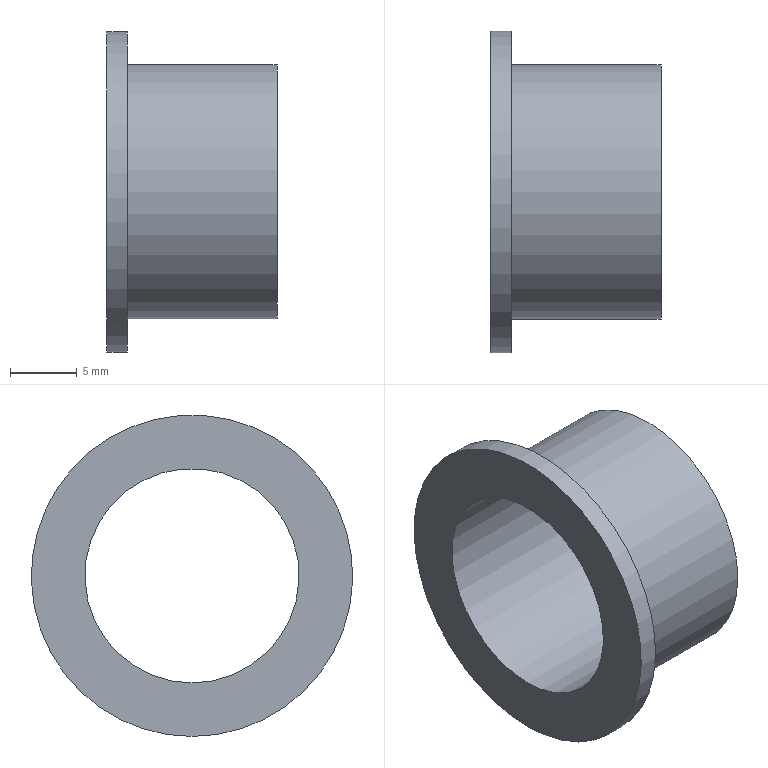Part | NX | features solid 2 | 1 solid | 6 faces | box 12.7 x 24 x 24 mm | volume 1301 mm3 | plane 3 | cylinder 3 | commonest cylinder face diameters 16 x1 19 x1 24 x1
STEP:
#1=CARTESIAN_POINT('',(0.,0.,-12.));
#2=VERTEX_POINT('',#1);
#3=CARTESIAN_POINT('',(0.,0.,0.));
#4=DIRECTION('',(1.,0.,0.));
#5=DIRECTION('',(0.,0.,-1.));
#6=AXIS2_PLACEMENT_3D('',#3,#4,#5);
#7=CIRCLE('',#6,12.);
#8=EDGE_CURVE('',#2,#2,#7,.T.);
#9=ORIENTED_EDGE('',*,*,#8,.F.);
#10=EDGE_LOOP('',(#9));
#11=FACE_BOUND('',#10,.T.);
#12=CARTESIAN_POINT('',(0.,0.,-8.));
#13=VERTEX_POINT('',#12);
#14=CARTESIAN_POINT('',(0.,0.,0.));
#15=DIRECTION('',(1.,0.,0.));
#16=DIRECTION('',(0.,0.,-1.));
#17=AXIS2_PLACEMENT_3D('',#14,#15,#16);
#18=CIRCLE('',#17,8.);
#19=EDGE_CURVE('',#13,#13,#18,.T.);
#20=ORIENTED_EDGE('',*,*,#19,.T.);
#21=EDGE_LOOP('',(#20));
#22=FACE_BOUND('',#21,.T.);
#23=CARTESIAN_POINT('',(0.,0.,8.));
#24=DIRECTION('',(1.,0.,0.));
#25=DIRECTION('',(0.,0.,-1.));
#26=AXIS2_PLACEMENT_3D('',#23,#24,#25);
#27=PLANE('',#26);
#28=ADVANCED_FACE('',(#11,#22),#27,.F.);
#29=CARTESIAN_POINT('',(1.5,0.,-12.));
#30=VERTEX_POINT('',#29);
#31=CARTESIAN_POINT('',(1.5,0.,0.));
#32=DIRECTION('',(1.,0.,0.));
#33=DIRECTION('',(0.,0.,-1.));
#34=AXIS2_PLACEMENT_3D('',#31,#32,#33);
#35=CIRCLE('',#34,12.);
#36=EDGE_CURVE('',#30,#30,#35,.T.);
#37=ORIENTED_EDGE('',*,*,#36,.F.);
#38=EDGE_LOOP('',(#37));
#39=FACE_BOUND('',#38,.T.);
#40=ORIENTED_EDGE('',*,*,#8,.T.);
#41=EDGE_LOOP('',(#40));
#42=FACE_BOUND('',#41,.T.);
#43=CARTESIAN_POINT('',(0.,0.,0.));
#44=DIRECTION('',(1.,0.,0.));
#45=DIRECTION('',(0.,0.,-1.));
#46=AXIS2_PLACEMENT_3D('',#43,#44,#45);
#47=CYLINDRICAL_SURFACE('',#46,12.);
#48=ADVANCED_FACE('',(#39,#42),#47,.T.);
#49=CARTESIAN_POINT('',(1.5,0.,-9.5));
#50=VERTEX_POINT('',#49);
#51=CARTESIAN_POINT('',(1.5,0.,0.));
#52=DIRECTION('',(1.,0.,0.));
#53=DIRECTION('',(0.,0.,-1.));
#54=AXIS2_PLACEMENT_3D('',#51,#52,#53);
#55=CIRCLE('',#54,9.5);
#56=EDGE_CURVE('',#50,#50,#55,.T.);
#57=ORIENTED_EDGE('',*,*,#56,.F.);
#58=EDGE_LOOP('',(#57));
#59=FACE_BOUND('',#58,.T.);
#60=ORIENTED_EDGE('',*,*,#36,.T.);
#61=EDGE_LOOP('',(#60));
#62=FACE_BOUND('',#61,.T.);
#63=CARTESIAN_POINT('',(1.5,0.,12.));
#64=DIRECTION('',(-1.,0.,0.));
#65=DIRECTION('',(0.,0.,1.));
#66=AXIS2_PLACEMENT_3D('',#63,#64,#65);
#67=PLANE('',#66);
#68=ADVANCED_FACE('',(#59,#62),#67,.F.);
#69=CARTESIAN_POINT('',(12.7,0.,-9.5));
#70=VERTEX_POINT('',#69);
#71=CARTESIAN_POINT('',(12.7,0.,0.));
#72=DIRECTION('',(1.,0.,0.));
#73=DIRECTION('',(0.,0.,-1.));
#74=AXIS2_PLACEMENT_3D('',#71,#72,#73);
#75=CIRCLE('',#74,9.5);
#76=EDGE_CURVE('',#70,#70,#75,.T.);
#77=ORIENTED_EDGE('',*,*,#76,.F.);
#78=EDGE_LOOP('',(#77));
#79=FACE_BOUND('',#78,.T.);
#80=ORIENTED_EDGE('',*,*,#56,.T.);
#81=EDGE_LOOP('',(#80));
#82=FACE_BOUND('',#81,.T.);
#83=CARTESIAN_POINT('',(0.,0.,0.));
#84=DIRECTION('',(1.,0.,0.));
#85=DIRECTION('',(0.,0.,-1.));
#86=AXIS2_PLACEMENT_3D('',#83,#84,#85);
#87=CYLINDRICAL_SURFACE('',#86,9.5);
#88=ADVANCED_FACE('',(#79,#82),#87,.T.);
#89=CARTESIAN_POINT('',(12.7,0.,-8.));
#90=VERTEX_POINT('',#89);
#91=CARTESIAN_POINT('',(12.7,0.,0.));
#92=DIRECTION('',(1.,0.,0.));
#93=DIRECTION('',(0.,0.,-1.));
#94=AXIS2_PLACEMENT_3D('',#91,#92,#93);
#95=CIRCLE('',#94,8.);
#96=EDGE_CURVE('',#90,#90,#95,.T.);
#97=ORIENTED_EDGE('',*,*,#96,.F.);
#98=EDGE_LOOP('',(#97));
#99=FACE_BOUND('',#98,.T.);
#100=ORIENTED_EDGE('',*,*,#76,.T.);
#101=EDGE_LOOP('',(#100));
#102=FACE_BOUND('',#101,.T.);
#103=CARTESIAN_POINT('',(12.7,0.,9.5));
#104=DIRECTION('',(-1.,0.,0.));
#105=DIRECTION('',(0.,0.,1.));
#106=AXIS2_PLACEMENT_3D('',#103,#104,#105);
#107=PLANE('',#106);
#108=ADVANCED_FACE('',(#99,#102),#107,.F.);
#109=ORIENTED_EDGE('',*,*,#19,.F.);
#110=EDGE_LOOP('',(#109));
#111=FACE_BOUND('',#110,.T.);
#112=ORIENTED_EDGE('',*,*,#96,.T.);
#113=EDGE_LOOP('',(#112));
#114=FACE_BOUND('',#113,.T.);
#115=CARTESIAN_POINT('',(0.,0.,0.));
#116=DIRECTION('',(1.,0.,0.));
#117=DIRECTION('',(0.,0.,-1.));
#118=AXIS2_PLACEMENT_3D('',#115,#116,#117);
#119=CYLINDRICAL_SURFACE('',#118,8.);
#120=ADVANCED_FACE('',(#111,#114),#119,.F.);
#121=CLOSED_SHELL('',(#28,#48,#68,#88,#108,#120));
#122=MANIFOLD_SOLID_BREP('',#121);
#123=(LENGTH_UNIT()NAMED_UNIT(*)SI_UNIT(.MILLI.,.METRE.));
#124=UNCERTAINTY_MEASURE_WITH_UNIT(LENGTH_MEASURE(0.00001),#123,'','');
#125=(NAMED_UNIT(*)PLANE_ANGLE_UNIT()SI_UNIT($,.RADIAN.));
#126=(NAMED_UNIT(*)SI_UNIT($,.STERADIAN.)SOLID_ANGLE_UNIT());
#127=(GEOMETRIC_REPRESENTATION_CONTEXT(3)GLOBAL_UNCERTAINTY_ASSIGNED_CONTEXT((#124))GLOBAL_UNIT_ASSIGNED_CONTEXT((#123,#125,#126))REPRESENTATION_CONTEXT('',''));
#128=ADVANCED_BREP_SHAPE_REPRESENTATION('',(#122),#127);